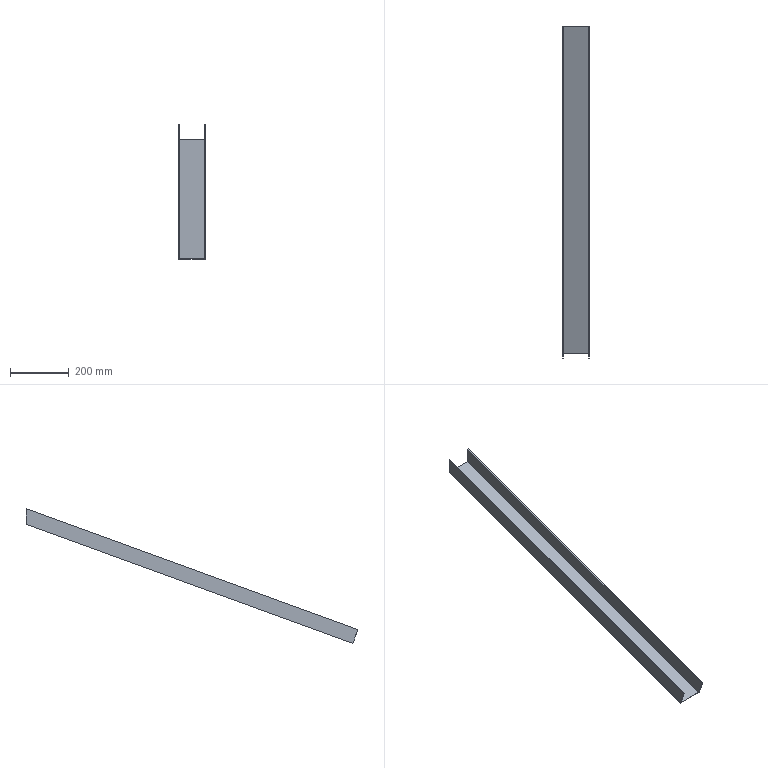Part | NX | features solid 2 | 1 solid | 10 faces | box 90 x 1127 x 457.216 mm | volume 441303 mm3 | plane 10
STEP:
#1=CARTESIAN_POINT('',(515.,85.,-106.054));
#2=VERTEX_POINT('',#1);
#3=CARTESIAN_POINT('',(517.,85.,-106.054));
#4=VERTEX_POINT('',#3);
#5=CARTESIAN_POINT('',(520.,85.,-106.054));
#6=DIRECTION('',(1.,0.,0.));
#7=VECTOR('',#6,1000.);
#8=LINE('',#5,#7);
#9=EDGE_CURVE('',#2,#4,#8,.T.);
#10=ORIENTED_EDGE('',*,*,#9,.T.);
#11=CARTESIAN_POINT('',(517.,85.,-157.135));
#12=VERTEX_POINT('',#11);
#13=CARTESIAN_POINT('',(517.,85.,-335.937));
#14=DIRECTION('',(0.,0.,-1.));
#15=VECTOR('',#14,1000.);
#16=LINE('',#13,#15);
#17=EDGE_CURVE('',#4,#12,#16,.T.);
#18=ORIENTED_EDGE('',*,*,#17,.T.);
#19=CARTESIAN_POINT('',(603.,85.,-157.135));
#20=VERTEX_POINT('',#19);
#21=CARTESIAN_POINT('',(520.,85.,-157.135));
#22=DIRECTION('',(1.,0.,0.));
#23=VECTOR('',#22,1000.);
#24=LINE('',#21,#23);
#25=EDGE_CURVE('',#12,#20,#24,.T.);
#26=ORIENTED_EDGE('',*,*,#25,.T.);
#27=CARTESIAN_POINT('',(603.,85.,-106.054));
#28=VERTEX_POINT('',#27);
#29=CARTESIAN_POINT('',(603.,85.,-80.));
#30=DIRECTION('',(0.,0.,-1.));
#31=VECTOR('',#30,1000.);
#32=LINE('',#29,#31);
#33=EDGE_CURVE('',#28,#20,#32,.T.);
#34=ORIENTED_EDGE('',*,*,#33,.F.);
#35=CARTESIAN_POINT('',(605.,85.,-106.054));
#36=VERTEX_POINT('',#35);
#37=CARTESIAN_POINT('',(520.,85.,-106.054));
#38=DIRECTION('',(1.,0.,0.));
#39=VECTOR('',#38,1000.);
#40=LINE('',#37,#39);
#41=EDGE_CURVE('',#28,#36,#40,.T.);
#42=ORIENTED_EDGE('',*,*,#41,.T.);
#43=CARTESIAN_POINT('',(605.,85.,-159.263));
#44=VERTEX_POINT('',#43);
#45=CARTESIAN_POINT('',(605.,85.,-80.));
#46=DIRECTION('',(0.,0.,-1.));
#47=VECTOR('',#46,1000.);
#48=LINE('',#45,#47);
#49=EDGE_CURVE('',#36,#44,#48,.T.);
#50=ORIENTED_EDGE('',*,*,#49,.T.);
#51=CARTESIAN_POINT('',(515.,85.,-159.263));
#52=VERTEX_POINT('',#51);
#53=CARTESIAN_POINT('',(520.,85.,-159.263));
#54=DIRECTION('',(1.,0.,0.));
#55=VECTOR('',#54,1000.);
#56=LINE('',#53,#55);
#57=EDGE_CURVE('',#52,#44,#56,.T.);
#58=ORIENTED_EDGE('',*,*,#57,.F.);
#59=CARTESIAN_POINT('',(515.,85.,-335.937));
#60=DIRECTION('',(0.,0.,-1.));
#61=VECTOR('',#60,1000.);
#62=LINE('',#59,#61);
#63=EDGE_CURVE('',#2,#52,#62,.T.);
#64=ORIENTED_EDGE('',*,*,#63,.F.);
#65=EDGE_LOOP('',(#10,#18,#26,#34,#42,#50,#58,#64));
#66=FACE_BOUND('',#65,.T.);
#67=CARTESIAN_POINT('',(-405.,85.,-80.));
#68=DIRECTION('',(0.,1.,0.));
#69=DIRECTION('',(-1.,0.,0.));
#70=AXIS2_PLACEMENT_3D('',#67,#68,#69);
#71=PLANE('',#70);
#72=ADVANCED_FACE('',(#66),#71,.T.);
#73=CARTESIAN_POINT('',(605.,-1042.101,-516.286));
#74=VERTEX_POINT('',#73);
#75=CARTESIAN_POINT('',(603.,-1042.101,-516.286));
#76=VERTEX_POINT('',#75);
#77=CARTESIAN_POINT('',(520.,-1042.101,-516.286));
#78=DIRECTION('',(-1.,0.,0.));
#79=VECTOR('',#78,1000.);
#80=LINE('',#77,#79);
#81=EDGE_CURVE('',#74,#76,#80,.T.);
#82=ORIENTED_EDGE('',*,*,#81,.T.);
#83=CARTESIAN_POINT('',(603.,-1025.684,-561.391));
#84=VERTEX_POINT('',#83);
#85=CARTESIAN_POINT('',(603.,-1042.101,-516.286));
#86=DIRECTION('',(0.,0.342,-0.9397));
#87=VECTOR('',#86,1000.);
#88=LINE('',#85,#87);
#89=EDGE_CURVE('',#76,#84,#88,.T.);
#90=ORIENTED_EDGE('',*,*,#89,.T.);
#91=CARTESIAN_POINT('',(517.,-1025.684,-561.391));
#92=VERTEX_POINT('',#91);
#93=CARTESIAN_POINT('',(520.,-1025.684,-561.391));
#94=DIRECTION('',(-1.,0.,0.));
#95=VECTOR('',#94,1000.);
#96=LINE('',#93,#95);
#97=EDGE_CURVE('',#84,#92,#96,.T.);
#98=ORIENTED_EDGE('',*,*,#97,.T.);
#99=CARTESIAN_POINT('',(517.,-1042.101,-516.286));
#100=VERTEX_POINT('',#99);
#101=CARTESIAN_POINT('',(517.,-1042.101,-516.286));
#102=DIRECTION('',(0.,0.342,-0.9397));
#103=VECTOR('',#102,1000.);
#104=LINE('',#101,#103);
#105=EDGE_CURVE('',#100,#92,#104,.T.);
#106=ORIENTED_EDGE('',*,*,#105,.F.);
#107=CARTESIAN_POINT('',(515.,-1042.101,-516.286));
#108=VERTEX_POINT('',#107);
#109=CARTESIAN_POINT('',(520.,-1042.101,-516.286));
#110=DIRECTION('',(-1.,0.,0.));
#111=VECTOR('',#110,1000.);
#112=LINE('',#109,#111);
#113=EDGE_CURVE('',#100,#108,#112,.T.);
#114=ORIENTED_EDGE('',*,*,#113,.T.);
#115=CARTESIAN_POINT('',(515.,-1025.,-563.27));
#116=VERTEX_POINT('',#115);
#117=CARTESIAN_POINT('',(515.,-1042.101,-516.286));
#118=DIRECTION('',(0.,0.342,-0.9397));
#119=VECTOR('',#118,1000.);
#120=LINE('',#117,#119);
#121=EDGE_CURVE('',#108,#116,#120,.T.);
#122=ORIENTED_EDGE('',*,*,#121,.T.);
#123=CARTESIAN_POINT('',(605.,-1025.,-563.27));
#124=VERTEX_POINT('',#123);
#125=CARTESIAN_POINT('',(520.,-1025.,-563.27));
#126=DIRECTION('',(-1.,0.,0.));
#127=VECTOR('',#126,1000.);
#128=LINE('',#125,#127);
#129=EDGE_CURVE('',#124,#116,#128,.T.);
#130=ORIENTED_EDGE('',*,*,#129,.F.);
#131=CARTESIAN_POINT('',(605.,-1042.101,-516.286));
#132=DIRECTION('',(0.,0.342,-0.9397));
#133=VECTOR('',#132,1000.);
#134=LINE('',#131,#133);
#135=EDGE_CURVE('',#74,#124,#134,.T.);
#136=ORIENTED_EDGE('',*,*,#135,.F.);
#137=EDGE_LOOP('',(#82,#90,#98,#106,#114,#122,#130,#136));
#138=FACE_BOUND('',#137,.T.);
#139=CARTESIAN_POINT('',(520.,-1042.101,-516.286));
#140=DIRECTION('',(0.,-0.9397,-0.342));
#141=DIRECTION('',(0.,0.342,-0.9397));
#142=AXIS2_PLACEMENT_3D('',#139,#140,#141);
#143=PLANE('',#142);
#144=ADVANCED_FACE('',(#138),#143,.T.);
#145=ORIENTED_EDGE('',*,*,#113,.F.);
#146=CARTESIAN_POINT('',(517.,-546.597,-335.937));
#147=DIRECTION('',(0.,0.9397,0.342));
#148=VECTOR('',#147,1000.);
#149=LINE('',#146,#148);
#150=EDGE_CURVE('',#100,#4,#149,.T.);
#151=ORIENTED_EDGE('',*,*,#150,.T.);
#152=ORIENTED_EDGE('',*,*,#9,.F.);
#153=CARTESIAN_POINT('',(515.,-546.597,-335.937));
#154=DIRECTION('',(0.,0.9397,0.342));
#155=VECTOR('',#154,1000.);
#156=LINE('',#153,#155);
#157=EDGE_CURVE('',#108,#2,#156,.T.);
#158=ORIENTED_EDGE('',*,*,#157,.F.);
#159=EDGE_LOOP('',(#145,#151,#152,#158));
#160=FACE_BOUND('',#159,.T.);
#161=CARTESIAN_POINT('',(520.,-546.597,-335.937));
#162=DIRECTION('',(0.,0.342,-0.9397));
#163=DIRECTION('',(-1.,0.,0.));
#164=AXIS2_PLACEMENT_3D('',#161,#162,#163);
#165=PLANE('',#164);
#166=ADVANCED_FACE('',(#160),#165,.F.);
#167=CARTESIAN_POINT('',(515.,-529.496,-382.921));
#168=DIRECTION('',(0.,0.9397,0.342));
#169=VECTOR('',#168,1000.);
#170=LINE('',#167,#169);
#171=EDGE_CURVE('',#116,#52,#170,.T.);
#172=ORIENTED_EDGE('',*,*,#171,.F.);
#173=ORIENTED_EDGE('',*,*,#121,.F.);
#174=ORIENTED_EDGE('',*,*,#157,.T.);
#175=ORIENTED_EDGE('',*,*,#63,.T.);
#176=EDGE_LOOP('',(#172,#173,#174,#175));
#177=FACE_BOUND('',#176,.T.);
#178=CARTESIAN_POINT('',(515.,-546.597,-335.937));
#179=DIRECTION('',(-1.,0.,0.));
#180=DIRECTION('',(0.,0.08716,0.9962));
#181=AXIS2_PLACEMENT_3D('',#178,#179,#180);
#182=PLANE('',#181);
#183=ADVANCED_FACE('',(#177),#182,.T.);
#184=CARTESIAN_POINT('',(605.,-529.496,-382.921));
#185=DIRECTION('',(0.,-0.9397,-0.342));
#186=VECTOR('',#185,1000.);
#187=LINE('',#184,#186);
#188=EDGE_CURVE('',#44,#124,#187,.T.);
#189=ORIENTED_EDGE('',*,*,#188,.F.);
#190=ORIENTED_EDGE('',*,*,#49,.F.);
#191=CARTESIAN_POINT('',(605.,-546.597,-335.937));
#192=DIRECTION('',(0.,-0.9397,-0.342));
#193=VECTOR('',#192,1000.);
#194=LINE('',#191,#193);
#195=EDGE_CURVE('',#36,#74,#194,.T.);
#196=ORIENTED_EDGE('',*,*,#195,.T.);
#197=ORIENTED_EDGE('',*,*,#135,.T.);
#198=EDGE_LOOP('',(#189,#190,#196,#197));
#199=FACE_BOUND('',#198,.T.);
#200=CARTESIAN_POINT('',(605.,-546.597,-335.937));
#201=DIRECTION('',(1.,0.,0.));
#202=DIRECTION('',(0.,-0.08716,-0.9962));
#203=AXIS2_PLACEMENT_3D('',#200,#201,#202);
#204=PLANE('',#203);
#205=ADVANCED_FACE('',(#199),#204,.T.);
#206=ORIENTED_EDGE('',*,*,#41,.F.);
#207=CARTESIAN_POINT('',(603.,-546.597,-335.937));
#208=DIRECTION('',(0.,-0.9397,-0.342));
#209=VECTOR('',#208,1000.);
#210=LINE('',#207,#209);
#211=EDGE_CURVE('',#28,#76,#210,.T.);
#212=ORIENTED_EDGE('',*,*,#211,.T.);
#213=ORIENTED_EDGE('',*,*,#81,.F.);
#214=ORIENTED_EDGE('',*,*,#195,.F.);
#215=EDGE_LOOP('',(#206,#212,#213,#214));
#216=FACE_BOUND('',#215,.T.);
#217=CARTESIAN_POINT('',(520.,-546.597,-335.937));
#218=DIRECTION('',(0.,0.342,-0.9397));
#219=DIRECTION('',(-1.,0.,0.));
#220=AXIS2_PLACEMENT_3D('',#217,#218,#219);
#221=PLANE('',#220);
#222=ADVANCED_FACE('',(#216),#221,.F.);
#223=ORIENTED_EDGE('',*,*,#171,.T.);
#224=ORIENTED_EDGE('',*,*,#57,.T.);
#225=ORIENTED_EDGE('',*,*,#188,.T.);
#226=ORIENTED_EDGE('',*,*,#129,.T.);
#227=EDGE_LOOP('',(#223,#224,#225,#226));
#228=FACE_BOUND('',#227,.T.);
#229=CARTESIAN_POINT('',(520.,-529.496,-382.921));
#230=DIRECTION('',(0.,0.342,-0.9397));
#231=DIRECTION('',(-1.,0.,0.));
#232=AXIS2_PLACEMENT_3D('',#229,#230,#231);
#233=PLANE('',#232);
#234=ADVANCED_FACE('',(#228),#233,.T.);
#235=CARTESIAN_POINT('',(517.,-530.18,-381.042));
#236=DIRECTION('',(0.,0.9397,0.342));
#237=VECTOR('',#236,1000.);
#238=LINE('',#235,#237);
#239=EDGE_CURVE('',#92,#12,#238,.T.);
#240=ORIENTED_EDGE('',*,*,#239,.T.);
#241=ORIENTED_EDGE('',*,*,#17,.F.);
#242=ORIENTED_EDGE('',*,*,#150,.F.);
#243=ORIENTED_EDGE('',*,*,#105,.T.);
#244=EDGE_LOOP('',(#240,#241,#242,#243));
#245=FACE_BOUND('',#244,.T.);
#246=CARTESIAN_POINT('',(517.,-546.597,-335.937));
#247=DIRECTION('',(-1.,0.,0.));
#248=DIRECTION('',(0.,0.08716,0.9962));
#249=AXIS2_PLACEMENT_3D('',#246,#247,#248);
#250=PLANE('',#249);
#251=ADVANCED_FACE('',(#245),#250,.F.);
#252=CARTESIAN_POINT('',(603.,-530.18,-381.042));
#253=DIRECTION('',(0.,-0.9397,-0.342));
#254=VECTOR('',#253,1000.);
#255=LINE('',#252,#254);
#256=EDGE_CURVE('',#20,#84,#255,.T.);
#257=ORIENTED_EDGE('',*,*,#256,.T.);
#258=ORIENTED_EDGE('',*,*,#89,.F.);
#259=ORIENTED_EDGE('',*,*,#211,.F.);
#260=ORIENTED_EDGE('',*,*,#33,.T.);
#261=EDGE_LOOP('',(#257,#258,#259,#260));
#262=FACE_BOUND('',#261,.T.);
#263=CARTESIAN_POINT('',(603.,-546.597,-335.937));
#264=DIRECTION('',(1.,0.,0.));
#265=DIRECTION('',(0.,-0.08716,-0.9962));
#266=AXIS2_PLACEMENT_3D('',#263,#264,#265);
#267=PLANE('',#266);
#268=ADVANCED_FACE('',(#262),#267,.F.);
#269=ORIENTED_EDGE('',*,*,#239,.F.);
#270=ORIENTED_EDGE('',*,*,#97,.F.);
#271=ORIENTED_EDGE('',*,*,#256,.F.);
#272=ORIENTED_EDGE('',*,*,#25,.F.);
#273=EDGE_LOOP('',(#269,#270,#271,#272));
#274=FACE_BOUND('',#273,.T.);
#275=CARTESIAN_POINT('',(520.,-530.18,-381.042));
#276=DIRECTION('',(0.,0.342,-0.9397));
#277=DIRECTION('',(-1.,0.,0.));
#278=AXIS2_PLACEMENT_3D('',#275,#276,#277);
#279=PLANE('',#278);
#280=ADVANCED_FACE('',(#274),#279,.F.);
#281=CLOSED_SHELL('',(#72,#144,#166,#183,#205,#222,#234,#251,#268,#280));
#282=MANIFOLD_SOLID_BREP('',#281);
#283=(LENGTH_UNIT()NAMED_UNIT(*)SI_UNIT(.MILLI.,.METRE.));
#284=UNCERTAINTY_MEASURE_WITH_UNIT(LENGTH_MEASURE(0.00001),#283,'','');
#285=(NAMED_UNIT(*)PLANE_ANGLE_UNIT()SI_UNIT($,.RADIAN.));
#286=(NAMED_UNIT(*)SI_UNIT($,.STERADIAN.)SOLID_ANGLE_UNIT());
#287=(GEOMETRIC_REPRESENTATION_CONTEXT(3)GLOBAL_UNCERTAINTY_ASSIGNED_CONTEXT((#284))GLOBAL_UNIT_ASSIGNED_CONTEXT((#283,#285,#286))REPRESENTATION_CONTEXT('',''));
#288=ADVANCED_BREP_SHAPE_REPRESENTATION('',(#282),#287);